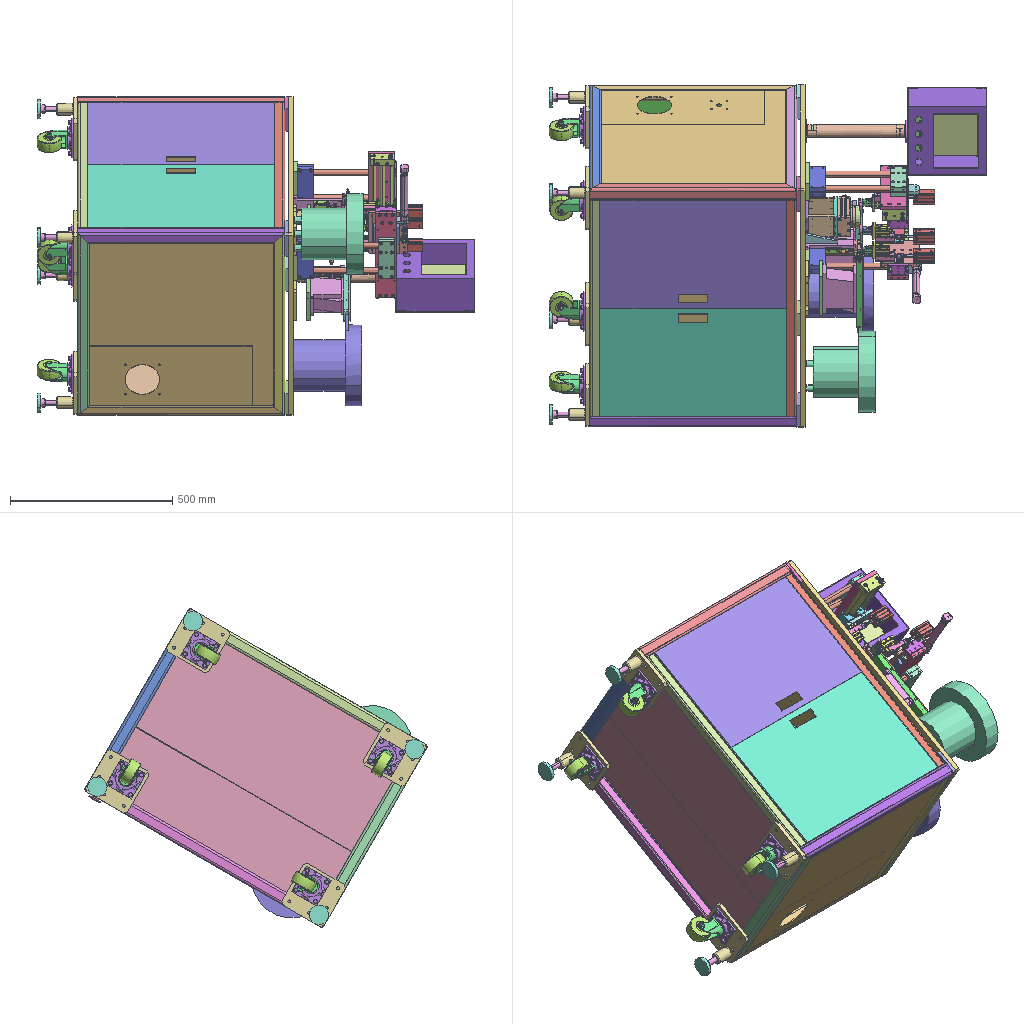Assembly | STEP file | 72 different items | 138 placed | box 1351 x 1056 x 983 mm
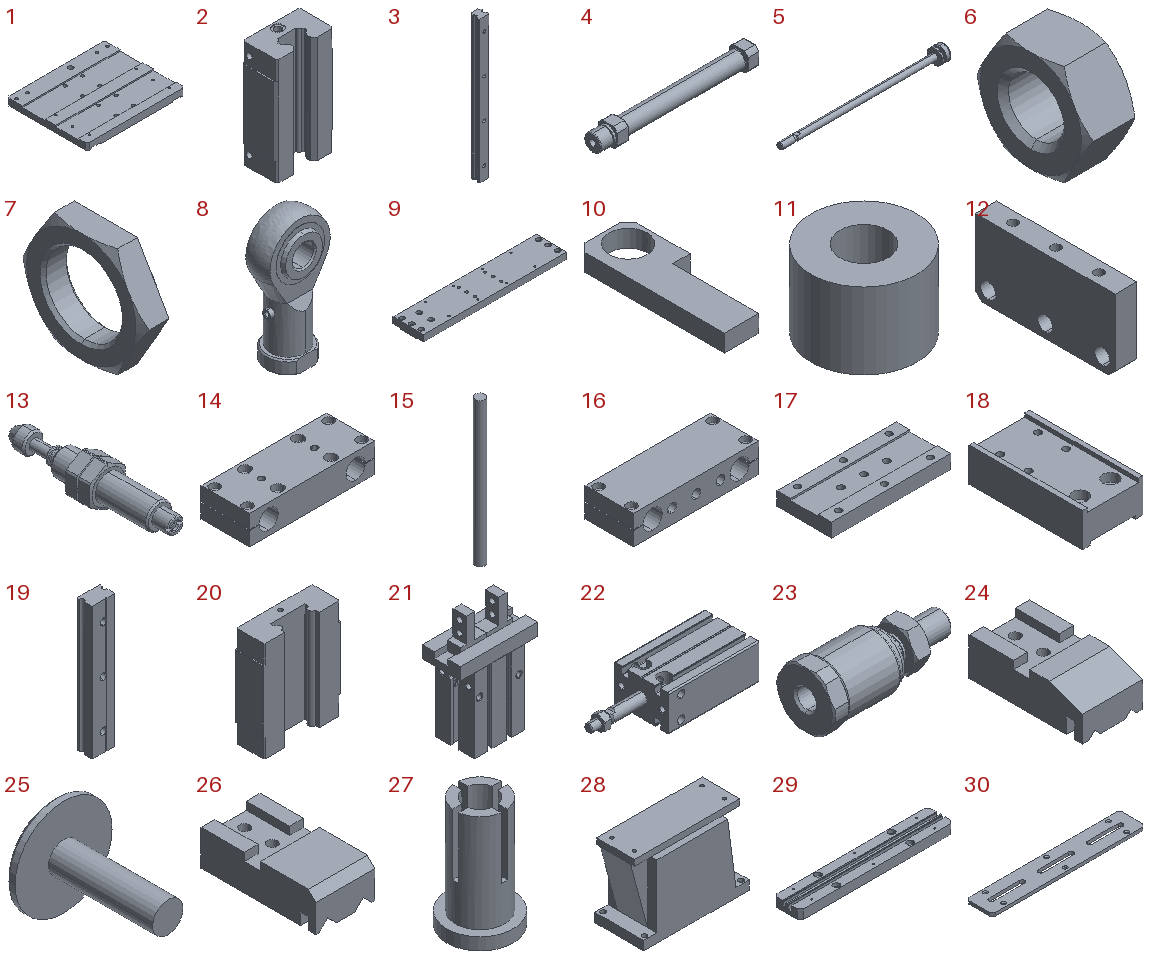Parts list (item | name | quantity | parent item | size | volume):
1 | A04 | x1 | in Feeding move | 146 x 120 x 10 mm | 149212 mm3
2 | HGH15_2 | x2 | in HGL15CA1R220 | 34 x 19.7 x 61.4 mm | 31145 mm3
3 | HGR15_1 | x2 | in HGL15CA1R220 | 15 x 15 x 220 mm | 40412 mm3
4 | _MI 20x125-S-U_c | x1 | in MI20x125SU | 207 x 25 x 25 mm | 36262 mm3
5 | _MI 20x125-S-U_r | x1 | in MI20x125SU | 216.2 x 19.5 x 19.5 mm | 13202 mm3
6 | _MI20-M8x1.25 - Nut | x1 | in MI20x125SU | 6 x 13.856 x 12 mm | 526.038 mm3
7 | _MI20-M22x1.5 - Nut | x1 | in MI20x125SU | 7 x 33.486 x 29 mm | 2690 mm3
8 | F-M8X125U | x1 | in Feeding move | - | 6721 mm3
9 | A07 | x1 | in Feeding move | 300 x 65 x 15 mm | 264705 mm3
10 | A08 | x1 | in Feeding move | 30 x 86 x 10 mm | 16393 mm3
11 | A09 | x1 | in Feeding move | 18 x 18 x 13 mm | 2622 mm3
12 | A10 | x2 | in Feeding move | 10 x 65 x 34 mm | 20344 mm3
13 | ACA0806 | x4 | in Feeding move | - | -
14 | A11 | x2 | in Feeding move, Discharge | 130 x 50 x 30 mm | 151680 mm3
15 | A12 | x4 | in Feeding move, Discharge | 20 x 20 x 300 mm | 94248 mm3
16 | A13 | x2 | in Feeding move, Discharge | 130 x 50 x 30 mm | 142890 mm3
17 | A14 | x2 | in Feeding move, Discharge | 130 x 60 x 15 mm | 104797 mm3
18 | A06 | x3 | in Feeding, Discharge | 32 x 60 x 18 mm | 26849 mm3
19 | MANIFOLD_SOLID_BREP_99 | x3 | in MGN12C1R70 | 12 x 8 x 70 mm | 5872 mm3
20 | MANIFOLD_SOLID_BREP_100 | x3 | in MGN12C1R70 | 27 x 10 x 34.7 mm | 7015 mm3
21 | MHZL2-16D2 | x3 | in Feeding, Discharge | - | -
22 | MD-20x20-S | x3 | in Feeding, Discharge | - | -
23 | F-M06100F | x3 | in Feeding, Discharge | 34.5 x 14.8 x 14 mm | 3405 mm3
24 | A05 | x5 | in Feeding transfer, Discharge | 15 x 28.2 x 9.4 mm | 3287 mm3
25 | Glue nail | x10 | in Feeding transfer, Glue nail feeding, Discharge | 8 x 10.617 x 8 mm | 110.388 mm3
26 | A05-1 | x2 | in Feeding transfer | 15 x 29.2 x 9 mm | 3438 mm3
27 | Glue plug | x7 | in Feeding transfer, Glue plug feeding, Discharge | 5.4 x 5.4 x 9 mm | 70.19 mm3
28 | Direct vibration | x2 | in Glue plug feeding, Glue nail feeding | 145 x 65 x 104 mm | 744100 mm3
29 | B01 | x1 | in Glue plug feeding | 250 x 43 x 15 mm | 136288 mm3
30 | B02 | x2 | in Glue plug feeding, Glue nail feeding | 250 x 43 x 5 mm | 46334 mm3
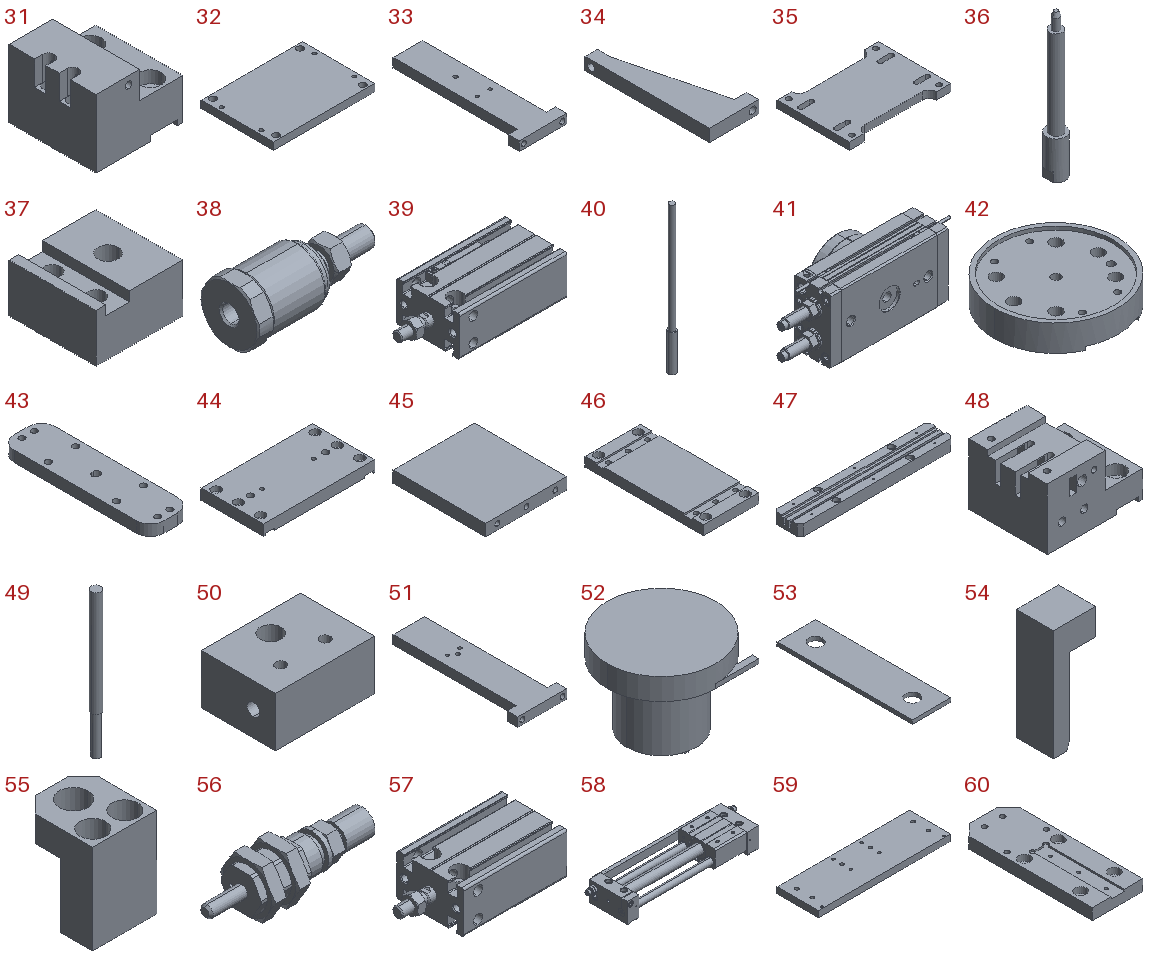31 | B03 | x1 | in Glue plug feeding | 32 x 32 x 25 mm | 18185 mm3
32 | B04 | x2 | in Glue plug feeding, Glue nail feeding | 140 x 100 x 10 mm | 136670 mm3
33 | B05 | x1 | in Glue plug feeding | 52 x 147 x 10 mm | 48382 mm3
34 | B06 | x2 | in Glue plug feeding, Glue nail feeding | 40 x 100 x 10 mm | 20525 mm3
35 | B07 | x2 | in Glue plug feeding, Glue nail feeding | 140 x 100 x 10 mm | 114178 mm3
36 | B09 | x3 | in Glue plug feeding | 6 x 6 x 45 mm | 663.346 mm3
37 | B10 | x1 | in Glue plug feeding | 18 x 18 x 10 mm | 2612 mm3
38 | F-M5X080F | x1 | in Glue plug feeding | 34.5 x 14.8 x 14 mm | 3243 mm3
39 | MD-16x15-S | x1 | in Glue plug feeding | - | -
40 | FU-49U | x4 | in Glue plug feeding, Glue nail feeding | 2 x 2 x 40 mm | 84.43 mm3
41 | HRQ30A | x1 | in Rotate | - | -
42 | C01 | x1 | in Rotate | 70 x 70 x 15 mm | 40707 mm3
43 | C02 | x2 | in Rotate | 30 x 110 x 8 mm | 23959 mm3
44 | C05 | x1 | in Rotate | 125 x 70 x 12 mm | 97826 mm3
45 | C06 | x2 | in Rotate | 70 x 80 x 10 mm | 54934 mm3
46 | C07 | x1 | in Rotate | 70 x 150 x 12 mm | 116800 mm3
47 | D01 | x1 | in Glue nail feeding | 250 x 43 x 18 mm | 165403 mm3
48 | D03 | x1 | in Glue nail feeding | 43 x 35 x 27.5 mm | 27305 mm3
49 | D05 | x2 | in Glue nail feeding | 2.5 x 2.5 x 37 mm | 163.952 mm3
50 | D06 | x1 | in Glue nail feeding | 20 x 15 x 10 mm | 2737 mm3
51 | D07 | x1 | in Glue nail feeding | 55 x 150 x 10 mm | 53842 mm3
52 | O-ring vibration plate | x1 | in Glue nail feeding | 250 x 250 x 210 mm | 5297074 mm3
53 | D04 | x1 | in Glue nail feeding | 10 x 35 x 1 mm | 330.758 mm3
54 | D09 | x2 | in Glue nail feeding | 8 x 7 x 21 mm | 572.033 mm3
55 | D10 | x2 | in Glue nail feeding | 20 x 23 x 28 mm | 4706 mm3
56 | CCOMPANY_AB6-5H4-B | x2 | in Glue nail feeding | - | -
57 | MD-16x10-S | x1 | in Glue nail feeding | - | -
58 | RMT16X150SA | x1 | in Discharge | - | -
59 | E01 | x1 | in Discharge | 257 x 80 x 12 mm | 241598 mm3
60 | E02 | x1 | in Discharge | 45 x 120 x 10 mm | 48925 mm3
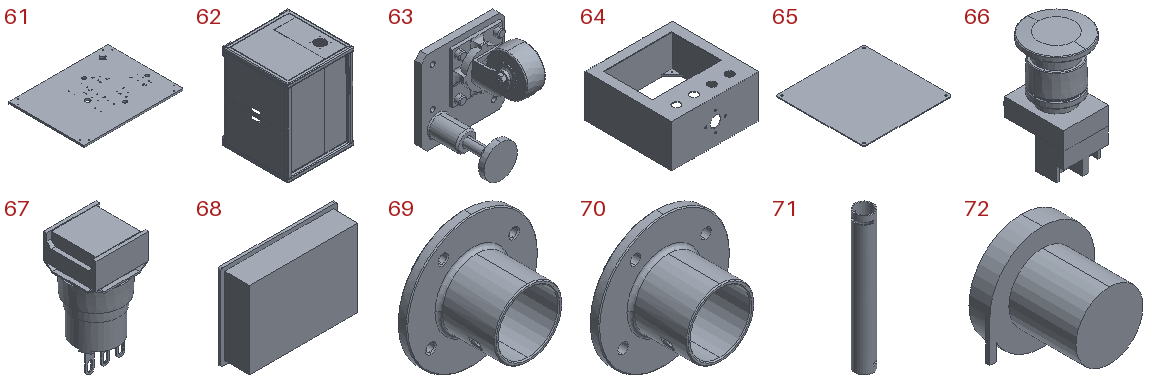61 | Base plate | x1 | in 37 | 850 x 650 x 15 mm | 8193242 mm3
62 | Frame_default<machined> | x1 | in Frame | 650 x 650 x 850 mm | 14326768 mm3
63 | CAL75 | x4 | in Frame | - | -
64 | Sheet metal box | x1 | in Touch screen | 245 x 245 x 120 mm | 296398 mm3
65 | Panel | x1 | in Touch screen | 240 x 240 x 2 mm | 114123 mm3
66 | Emergency stop | x1 | in Touch screen | 39.8 x 41.5 x 73.6 mm | 50842 mm3
67 | Button | x4 | in Touch screen | 18.8 x 18.8 x 38.3 mm | 7439 mm3
68 | Weinview-MT506MV5 | x1 | in Touch screen | 204 x 48.75 x 150 mm | 1264781 mm3
69 | Support base | x1 | in Touch screen | 70 x 35 x 70 mm | 21236 mm3
70 | Support base1 | x1 | in Touch screen | 70 x 35 x 70 mm | 21049 mm3
71 | Support tube | x1 | in Touch screen | 40 x 40 x 300 mm | 70315 mm3
72 | Vibration plate3 | x1 | in 37 | 250 x 210 x 250 mm | 5680348 mm3
Placements (level | parent | child | x y z in mm | rotation matrix by rows):
1 | 37 | Feeding transfer | 4.931 181.422 -23.15 | 0 1 0 0.5 0 -0.866 -0.866 0 -0.5
2 | Feeding transfer | Feeding move | -0.0 -0.0 -0.0 | 1 0 0 0 1 0 0 0 1
3 | Feeding move | A04 | -0.0 -0.0 -0.0 | 1 0 0 0 1 0 0 0 1
3 | Feeding move | HGL15CA1R220 | -0.0 20.0 17.0 | 0 0 1 -1 0 0 0 -1 -0
4 | HGL15CA1R220 | HGH15_2 | -0.0 -0.0 -0.0 | 1 0 0 0 1 0 0 0 1
4 | HGL15CA1R220 | HGR15_1 | -0.0 -0.0 30.0 | 1 0 0 0 1 0 0 0 1
3 | Feeding move | HGL15CA1R220 | -0.0 -30.0 17.0 | 0 0 1 -1 0 0 0 -1 -0
4 | HGL15CA1R220 | HGH15_2 | -0.0 -0.0 -0.0 | 1 0 0 0 1 0 0 0 1
4 | HGL15CA1R220 | HGR15_1 | -0.0 -0.0 30.0 | 1 0 0 0 1 0 0 0 1
3 | Feeding move | MI20x125SU | -60.0 50.5 29.0 | -1 0 0 0 1 0 0 0 -1
4 | MI20x125SU | _MI 20x125-S-U_c | 0.0 -0.0 -0.0 | 1 0 0 0 1 0 0 0 1
4 | MI20x125SU | _MI 20x125-S-U_r | -2.0 0.0 -0.0 | 1 0 0 0 1 0 0 0 1
4 | MI20x125SU | _MI20-M8x1.25 - Nut | -37.0 0.0 -0.0 | 1 0 0 0 1 0 0 0 1
4 | MI20x125SU | _MI20-M22x1.5 - Nut | -17.0 0.0 0.0 | 1 0 0 0 0.866 -0.5 0 0.5 0.866
3 | Feeding move | F-M8X125U | -23.0 50.5 29.0 | 0 0 1 -1 0 0 0 -1 -0
3 | Feeding move | A07 | 60.0 -5.0 30.0 | 1 0 0 0 1 0 0 0 1
3 | Feeding move | A08 | -50.0 20.5 27.0 | 0 0 -1 0 1 0 1 0 0
3 | Feeding move | A09 | 13.0 50.5 10.0 | 1 0 0 0 1 0 0 0 1
3 | Feeding move | A10 | -83.0 -5.0 -2.0 | 1 0 0 0 1 0 0 0 1
3 | Feeding move | ACA0806 | -117.0 21.5 4.0 | 0 1 0 -0.9106 0 0.4133 0.4133 0 0.9106
3 | Feeding move | A10 | 203.0 -5.0 -2.0 | 1 0 0 0 1 0 0 0 1
3 | Feeding move | ACA0806 | -117.0 -31.5 4.0 | 0 1 0 -1 0 0 0 0 1
3 | Feeding move | ACA0806 | 237.0 21.5 4.0 | 0 -1 0 1 0 0 0 0 1
3 | Feeding move | ACA0806 | 237.0 -31.5 4.0 | 0 -1 0 1 0 0 0 0 1
3 | Feeding move | A11 | 60.0 -5.0 45.0 | 1 0 0 0 1 0 0 0 1
3 | Feeding move | A12 | 15.0 -280.0 60.0 | 1 0 0 0 0 1 0 -1 -0
3 | Feeding move | A12 | 105.0 -280.0 60.0 | 1 0 0 0 0 1 0 -1 -0
3 | Feeding move | A13 | 60.0 -255.0 45.0 | 1 0 0 0 1 0 0 0 1
3 | Feeding move | A14 | 60.0 -293.0 60.0 | 1 0 0 0 0 1 0 -1 -0
2 | Feeding transfer | Feeding | -127.3 -69.105 -42.962 | 0 0 1 1 0 0 0 1 0
3 | Feeding | A06 | 22.105 15.462 67.3 | 0 1 0 0 0 1 1 0 0
3 | Feeding | MGN12C1R70 | 44.105 44.462 67.3 | 0 0 1 0 -1 0 1 0 -0
4 | MGN12C1R70 | MANIFOLD_SOLID_BREP_99 | 0.0 0.0 -0.0 | 1 0 0 0 1 0 0 0 1
4 | MGN12C1R70 | MANIFOLD_SOLID_BREP_100 | 0.0 0.0 -10.0 | 1 0 0 0 1 0 0 0 1
3 | Feeding | MHZL2-16D2 | 37.304 1.962 67.3 | 0 0 -1 -1 0 0 0 1 0
3 | Feeding | MD-20x20-S | 110.605 22.962 67.3 | 1 0 0 0 -1 0 0 0 -1
3 | Feeding | F-M06100F | 78.605 22.962 67.3 | -1 0 0 0 0.3818 -0.9242 0 -0.9242 -0.3818
2 | Feeding transfer | A05 | -60.0 -100.9 -41.05 | -1 0 0 0 1 0 0 0 -1
2 | Feeding transfer | A05 | -60.0 -100.9 -40.95 | 1 0 0 0 1 0 0 0 1
2 | Feeding transfer | Glue nail | -55.5 -111.0 -41.0 | 0.9984 0 0.05664 0 1 0 -0.05664 0 0.9984
2 | Feeding transfer | Glue nail | -64.5 -111.0 -41.0 | 0.9984 0 0.05664 0 1 0 -0.05664 0 0.9984
2 | Feeding transfer | Feeding | -7.3 -69.105 -42.962 | 0 0 1 1 0 0 0 1 0
3 | Feeding | A06 | 22.105 15.462 67.3 | 0 1 0 0 0 1 1 0 0
3 | Feeding | MGN12C1R70 | 44.105 44.462 67.3 | 0 0 1 0 -1 0 1 0 -0
4 | MGN12C1R70 | MANIFOLD_SOLID_BREP_99 | 0.0 0.0 -0.0 | 1 0 0 0 1 0 0 0 1
4 | MGN12C1R70 | MANIFOLD_SOLID_BREP_100 | 0.0 0.0 -10.0 | 1 0 0 0 1 0 0 0 1
3 | Feeding | MHZL2-16D2 | 37.304 1.962 67.3 | 0 0 -1 -1 0 0 0 1 0
3 | Feeding | MD-20x20-S | 110.605 22.962 67.3 | 1 0 0 0 -1 0 0 0 -1
3 | Feeding | F-M06100F | 78.605 22.962 67.3 | -1 0 0 0 0.3818 -0.9242 0 -0.9242 -0.3818
2 | Feeding transfer | A05-1 | 60.0 -101.4 -41.45 | -1 0 0 0 1 0 0 0 -1
2 | Feeding transfer | A05-1 | 60.0 -101.4 -40.55 | 1 0 0 0 1 0 0 0 1
2 | Feeding transfer | Glue plug | 64.5 -113.0 -41.0 | -0.9959 -0.09008 0 0 0 -1 0.09008 -0.9959 -0
2 | Feeding transfer | Glue plug | 55.5 -113.0 -41.0 | -0.9959 -0.09008 0 0 0 -1 0.09008 -0.9959 -0
2 | Feeding transfer | Glue plug | 184.5 -113.0 -41.0 | -0.9959 -0.09008 0 0 0 -1 0.09008 -0.9959 -0
2 | Feeding transfer | Glue plug | 175.5 -113.0 -41.0 | -0.9959 -0.09008 0 0 0 -1 0.09008 -0.9959 -0
2 | Feeding transfer | A05 | -60.0 -100.9 -34.95 | 1 0 0 0 1 0 0 0 1
1 | 37 | Glue plug feeding | -319.569 200.816 -217.069 | 0 0 1 0.866 -0.5 0 0.5 0.866 0
2 | Glue plug feeding | Direct vibration | -2.837 -2.364 84.0 | 1 0 0 0 1 0 0 0 1
2 | Glue plug feeding | B01 | -7.837 -2.364 188.0 | 1 0 0 0 1 0 0 0 1
2 | Glue plug feeding | B02 | -7.837 -2.364 203.0 | 1 0 0 0 1 0 0 0 1
2 | Glue plug feeding | B03 | 134.163 -2.364 176.5 | 1 0 0 0 1 0 0 0 1
2 | Glue plug feeding | B04 | -2.837 -2.364 74.0 | 1 0 0 0 1 0 0 0 1
2 | Glue plug feeding | B05 | 148.163 -2.364 105.0 | 0 0 -1 -1 0 0 0 1 0
2 | Glue plug feeding | B06 | 168.163 2.636 81.5 | 1 0 0 0 0 -1 0 1 0
2 | Glue plug feeding | B07 | -2.837 -2.364 31.5 | 1 0 0 0 1 0 0 0 1
2 | Glue plug feeding | Glue plug | 121.163 -6.864 202.5 | -0.9716 -0.2365 0 -0.2365 0.9716 0 0 0 -1
2 | Glue plug feeding | B09 | 121.163 -6.864 159.5 | 1 0 0 0 1 0 0 0 1
2 | Glue plug feeding | B09 | 121.163 2.136 159.5 | 1 0 0 0 1 0 0 0 1
2 | Glue plug feeding | B10 | 125.663 -2.364 139.5 | 1 0 0 0 1 0 0 0 1
2 | Glue plug feeding | F-M5X080F | 128.163 -2.364 113.0 | 0 0 -1 0 1 0 1 0 0
2 | Glue plug feeding | MD-16x15-S | 128.163 -2.364 103.0 | 0 0 1 0 1 0 -1 0 -0
2 | Glue plug feeding | B09 | 121.163 -6.864 174.5 | 1 0 0 0 1 0 0 0 1
2 | Glue plug feeding | FU-49U | 124.163 -6.864 198.5 | 0 0 1 0 1 0 -1 0 0
2 | Glue plug feeding | FU-49U | 124.163 2.136 198.5 | 0 0 1 0 1 0 -1 0 0
1 | 37 | Rotate | -188.069 290.23 -29.611 | 0 1 0 -0.5 0 0.866 0.866 0 0.5
2 | Rotate | HRQ30A | -0.0 -0.0 -0.0 | 1 0 0 0 1 0 0 0 1
2 | Rotate | C01 | -0.0 70.0 -0.0 | 1 0 0 0 0 -1 0 1 0
2 | Rotate | C02 | -0.0 76.0 0.0 | 1 0 0 0 0 -1 0 1 0
2 | Rotate | C05 | -0.0 -12.0 -0.0 | 1 0 0 0 0 1 0 -1 0
2 | Rotate | C06 | 60.5 -50.0 -0.0 | 0 0 -1 0 1 0 1 0 0
2 | Rotate | C06 | -50.5 -50.0 -0.0 | 0 0 -1 0 1 0 1 0 0
2 | Rotate | C07 | 0.0 -100.0 -0.0 | 0 -1 0 0 0 1 -1 0 0
2 | Rotate | C02 | 0.0 76.0 -0.0 | -0.7071 0.7071 0 0 0 -1 -0.7071 -0.7071 0
1 | 37 | Glue nail feeding | -317.069 69.707 -25.463 | 0 0 1 0.866 -0.5 0 0.5 0.866 -0
2 | Glue nail feeding | Direct vibration | 3.404 6.146 83 | 1 0 0 0 1 0 0 0 1
2 | Glue nail feeding | D01 | -1.596 6.146 187 | 1 0 0 0 1 0 0 0 1
2 | Glue nail feeding | B04 | 3.404 6.146 73 | 1 0 0 0 1 0 0 0 1
2 | Glue nail feeding | B07 | 3.404 6.146 29.5 | 1 0 0 0 1 0 0 0 1
2 | Glue nail feeding | D03 | 137.404 6.146 177.5 | 1 0 0 0 1 0 0 0 1
2 | Glue nail feeding | D05 | 138.904 1.646 162.9 | -0.9599 -0.2803 0 0.2803 -0.9599 0 0 0 1
2 | Glue nail feeding | D06 | 141.904 6.146 152.9 | 0 1 0 -1 0 0 0 0 1
2 | Glue nail feeding | D07 | 155.404 6.146 104.5 | 0 0 1 1 0 0 0 1 0
2 | Glue nail feeding | B06 | 185.404 11.146 79.5 | 1 0 0 0 0 -1 0 1 0
2 | Glue nail feeding | O-ring vibration plate | -226.596 123.646 55 | 1 0 0 0 1 0 0 0 1
2 | Glue nail feeding | Glue nail | 138.904 1.646 204.5 | 0.09915 0 0.9951 0.9951 0 -0.09915 0 1 0
2 | Glue nail feeding | Glue nail | 138.904 10.646 204.5 | 0.09915 0 0.9951 0.9951 0 -0.09915 0 1 0
2 | Glue nail feeding | Glue nail | 138.904 10.646 211 | 0.09915 0 0.9951 0.9951 0 -0.09915 0 1 0
2 | Glue nail feeding | Glue nail | 138.904 1.646 211 | 0.09915 0 0.9951 0.9951 0 -0.09915 0 1 0
2 | Glue nail feeding | D04 | 129.404 6.146 205 | 1 0 0 0 1 0 0 0 1
2 | Glue nail feeding | Glue nail | 130.904 10.646 204.5 | 0.09915 0 0.9951 0.9951 0 -0.09915 0 1 0
2 | Glue nail feeding | Glue nail | 130.904 1.646 204.5 | 0.09915 0 0.9951 0.9951 0 -0.09915 0 1 0
2 | Glue nail feeding | D09 | 136.104 4.646 198.5 | 1 0 0 0 0 -1 0 1 -0
2 | Glue nail feeding | D09 | 136.104 7.646 198.5 | 1 0 0 0 0 1 0 -1 0
2 | Glue nail feeding | D10 | 136.104 -11.354 193.5 | 1 0 0 0 0 -1 0 1 -0
2 | Glue nail feeding | CCOMPANY_AB6-5H4-B | 136.104 -30.354 198 | 0 1 0 -1 0 0 0 0 1
2 | Glue nail feeding | D10 | 136.104 23.646 193.5 | -1 0 0 0 0 1 0 1 0
2 | Glue nail feeding | CCOMPANY_AB6-5H4-B | 136.104 42.646 198 | 0 -0.8372 -0.5469 1 0 0 0 -0.5469 0.8372
2 | Glue nail feeding | D05 | 138.904 10.646 162.9 | -0.9599 -0.2803 0 0.2803 -0.9599 0 0 0 1
2 | Glue nail feeding | MD-16x10-S | 145.404 6.146 142.9 | 0 0 1 0 1 0 -1 0 0
2 | Glue nail feeding | B02 | -1.596 6.146 205 | 1 0 0 0 1 0 0 0 1
2 | Glue nail feeding | FU-49U | 140.404 1.646 200 | 0 0 1 0 1 0 -1 0 0
2 | Glue nail feeding | FU-49U | 140.404 10.646 200 | 0 0 1 -0.2359 0.9718 0 -0.9718 -0.2359 0
1 | 37 | Discharge | 10.374 584.246 279.149 | 0 1 0 0.5 0 -0.866 -0.866 0 -0.5
2 | Discharge | RMT16X150SA | -83.113 -22.943 287.506 | 1 0 0 0 1 0 0 0 1
2 | Discharge | E01 | 45.387 -25.443 256.006 | 1 0 0 0 1 0 0 0 1
2 | Discharge | E02 | 120.387 -5.943 308.006 | 1 0 0 0 1 0 0 0 1
2 | Discharge | MGN12C1R70 | 120.387 -30.943 316.506 | -1 0 0 0 0 1 0 1 0
3 | MGN12C1R70 | MANIFOLD_SOLID_BREP_99 | 0.0 0.0 -0.0 | 1 0 0 0 1 0 0 0 1
3 | MGN12C1R70 | MANIFOLD_SOLID_BREP_100 | 0.0 0.0 -10.0 | 1 0 0 0 1 0 0 0 1
2 | Discharge | A06 | 120.387 -52.943 345.506 | -1 0 0 0 1 0 0 0 -1
2 | Discharge | A11 | 45.387 -10.443 256.006 | -1 0 0 0 1 0 0 0 -1
2 | Discharge | A12 | 90.387 -285.443 241.006 | 1 0 0 0 0 1 0 -1 0
2 | Discharge | A12 | 0.3866 -285.443 241.006 | 1 0 0 0 0 1 0 -1 0
2 | Discharge | A13 | 45.387 -260.443 226.006 | 1 0 0 0 1 0 0 0 1
2 | Discharge | A14 | 45.387 -298.443 241.006 | 1 0 0 0 0 1 0 -1 0
2 | Discharge | MHZL2-16D2 | 120.387 -37.743 359.006 | 0 1 0 0 0 -1 -1 0 0
2 | Discharge | A05 | 120.387 -106.843 359.056 | 1 0 0 0 1 0 0 0 1
2 | Discharge | A05 | 120.387 -106.843 358.956 | -1 0 0 0 1 0 0 0 -1
2 | Discharge | Glue nail | 124.887 -116.943 359.006 | 1 0 0 0 1 0 0 0 1
2 | Discharge | Glue plug | 124.887 -121.943 359.006 | 1 0 0 0 0 -1 0 1 0
2 | Discharge | Glue nail | 115.887 -116.943 359.006 | 1 0 0 0 1 0 0 0 1
2 | Discharge | Glue plug | 115.887 -121.943 359.006 | 1 0 0 0 0 -1 0 1 0
2 | Discharge | F-M06100F | 120.387 3.557 338.006 | 0 1 0 -1 0 0 0 0 1
2 | Discharge | MD-20x20-S | 120.387 35.557 338.006 | 0 0 1 1 0 0 0 1 0
1 | 37 | Base plate | -288.069 168.987 -99.611 | 0 0 -1 0.866 0.5 0 0.5 -0.866 0
1 | 37 | Frame | -671.506 919.975 299.638 | 0 1 0 0.5 0 -0.866 -0.866 0 -0.5
2 | Frame | Frame_default<machined> | -334.734 -261.563 445.0 | 1 0 0 0 1 0 0 0 1
2 | Frame | CAL75 | -279.734 -281.563 500.0 | 1 0 0 0 1 0 0 0 1
2 | Frame | CAL75 | 220.266 -281.563 500.0 | 0 0 -1 0 1 0 1 0 0
2 | Frame | CAL75 | -279.734 -281.563 1200.0 | 0 0 1 0 1 0 -1 0 0
2 | Frame | CAL75 | 220.266 -281.563 1200.0 | -1 0 0 0 1 0 0 0 -1
1 | 37 | Touch screen | 34.086 623.265 57.815 | 0 1 0 -0.866 0 -0.5 -0.5 0 0.866
2 | Touch screen | Sheet metal box | 353.317 -215.826 -674.763 | 1 0 0 0 1 0 0 0 1
2 | Touch screen | Panel | 353.317 -215.826 -672.763 | 1 0 0 0 1 0 0 0 1
2 | Touch screen | Emergency stop | 195.63 45.345 -239.796 | 0 -1 0 -1 0 0 0 0 -1
2 | Touch screen | Button | 243.63 49.345 -211.996 | 0 -1 0 -1 0 0 0 0 -1
2 | Touch screen | Button | 203.63 49.345 -211.996 | 0 -1 0 -1 0 0 0 0 -1
2 | Touch screen | Button | 163.63 49.345 -211.996 | 0 -1 0 -1 0 0 0 0 -1
2 | Touch screen | Button | 123.63 49.345 -211.996 | 0 -1 0 -1 0 0 0 0 -1
2 | Touch screen | Weinview-MT506MV5 | -1142.493 -800.31 -340.434 | 1 0 0 0 0 1 0 -1 0
2 | Touch screen | Support base | -325.205 -223.655 -155.026 | -0.5736 0 0.8192 0 1 0 -0.8192 0 -0.5736
2 | Touch screen | Support base1 | 169.8 -104.655 -650.031 | -0.8192 0 -0.5736 0 -1 0 -0.5736 0 0.8192
2 | Touch screen | Support tube | 169.63 -164.155 -155.196 | 0.7144 -0.6997 0 0 0 -1 0.6997 0.7144 -0
1 | 37 | Vibration plate3 | -286.569 59.106 -437.292 | 0 1 0 0.5 0 -0.866 -0.866 0 -0.5